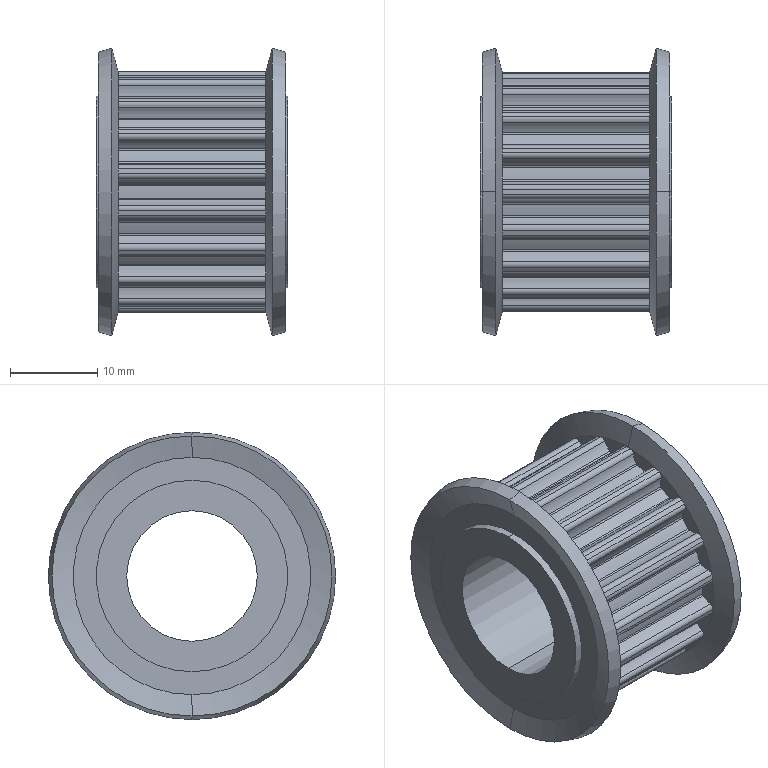Part | SolidWorks | 1 solid | 203 faces | box 22 x 33 x 33 mm | volume 8275 mm3 | cylinder 151 | plane 40 | cone 12 | commonest cylinder face diameters 0.5 x36 1.1 x36 6.55 x36 27.69 x19 24.15 x18 22 x4